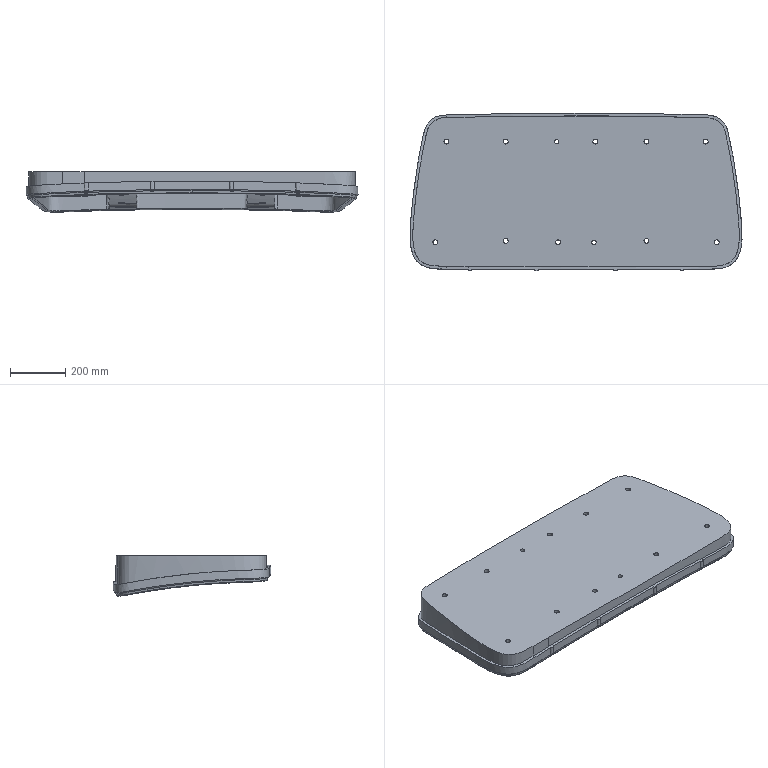Part | NX | features solid 2 | 1 solid | 297 faces | box 1204 x 571.61 x 146.904 mm | volume 43125275 mm3 | plane 121 | spline 102 | cylinder 64 | sphere 10 | commonest cylinder face diameters 6 x28 17.5 x10 25.5 x10 16 x6 6.004 x4 6.003 x2